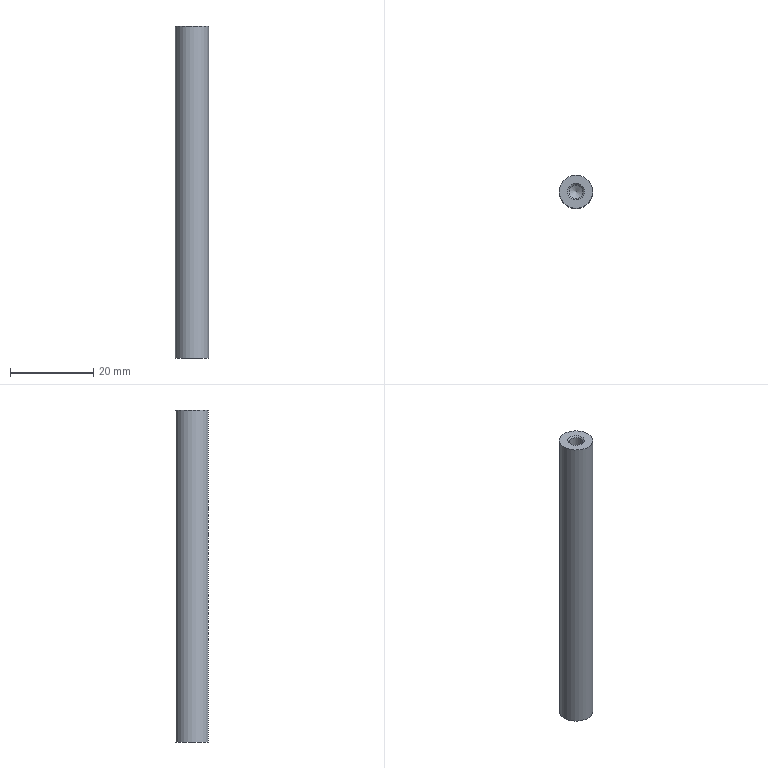Part | NX | features DATUM_CSYS 2, HOLE PACKAGE 2, SIMPLE HOLE 2, SYMBOLIC_THREAD 2, EXTRUDE 1, SKETCH 1 | 1 solid | 9 faces | box 8 x 8 x 80 mm | volume 3672 mm3 | cone 4 | cylinder 3 | plane 2 | commonest cylinder face diameters 3.3 x2 8 x1
STEP:
#1=CARTESIAN_POINT('',(4.,0.,80.));
#2=VERTEX_POINT('',#1);
#3=CARTESIAN_POINT('',(0.,0.,80.));
#4=DIRECTION('',(0.,0.,1.));
#5=DIRECTION('',(1.,0.,0.));
#6=AXIS2_PLACEMENT_3D('',#3,#4,#5);
#7=CIRCLE('',#6,4.);
#8=EDGE_CURVE('',#2,#2,#7,.T.);
#9=ORIENTED_EDGE('',*,*,#8,.F.);
#10=EDGE_LOOP('',(#9));
#11=FACE_BOUND('',#10,.T.);
#12=CARTESIAN_POINT('',(4.,0.,0.));
#13=VERTEX_POINT('',#12);
#14=CARTESIAN_POINT('',(0.,0.,0.));
#15=DIRECTION('',(0.,0.,1.));
#16=DIRECTION('',(1.,0.,0.));
#17=AXIS2_PLACEMENT_3D('',#14,#15,#16);
#18=CIRCLE('',#17,4.);
#19=EDGE_CURVE('',#13,#13,#18,.T.);
#20=ORIENTED_EDGE('',*,*,#19,.T.);
#21=EDGE_LOOP('',(#20));
#22=FACE_BOUND('',#21,.T.);
#23=CARTESIAN_POINT('',(0.,0.,80.));
#24=DIRECTION('',(0.,0.,-1.));
#25=DIRECTION('',(-1.,0.,0.));
#26=AXIS2_PLACEMENT_3D('',#23,#24,#25);
#27=CYLINDRICAL_SURFACE('',#26,4.);
#28=ADVANCED_FACE('',(#11,#22),#27,.T.);
#29=CARTESIAN_POINT('',(2.,0.,80.));
#30=VERTEX_POINT('',#29);
#31=CARTESIAN_POINT('',(0.,0.,80.));
#32=DIRECTION('',(0.,0.,1.));
#33=DIRECTION('',(1.,0.,0.));
#34=AXIS2_PLACEMENT_3D('',#31,#32,#33);
#35=CIRCLE('',#34,2.);
#36=EDGE_CURVE('',#30,#30,#35,.F.);
#37=ORIENTED_EDGE('',*,*,#36,.T.);
#38=EDGE_LOOP('',(#37));
#39=FACE_BOUND('',#38,.T.);
#40=ORIENTED_EDGE('',*,*,#8,.T.);
#41=EDGE_LOOP('',(#40));
#42=FACE_BOUND('',#41,.T.);
#43=CARTESIAN_POINT('',(0.,0.,80.));
#44=DIRECTION('',(0.,0.,1.));
#45=DIRECTION('',(1.,0.,0.));
#46=AXIS2_PLACEMENT_3D('',#43,#44,#45);
#47=PLANE('',#46);
#48=ADVANCED_FACE('',(#39,#42),#47,.T.);
#49=CARTESIAN_POINT('',(2.,0.,0.));
#50=VERTEX_POINT('',#49);
#51=CARTESIAN_POINT('',(0.,0.,0.));
#52=DIRECTION('',(0.,0.,1.));
#53=DIRECTION('',(1.,0.,0.));
#54=AXIS2_PLACEMENT_3D('',#51,#52,#53);
#55=CIRCLE('',#54,2.);
#56=EDGE_CURVE('',#50,#50,#55,.T.);
#57=ORIENTED_EDGE('',*,*,#56,.T.);
#58=EDGE_LOOP('',(#57));
#59=FACE_BOUND('',#58,.T.);
#60=ORIENTED_EDGE('',*,*,#19,.F.);
#61=EDGE_LOOP('',(#60));
#62=FACE_BOUND('',#61,.T.);
#63=CARTESIAN_POINT('',(0.,0.,0.));
#64=DIRECTION('',(0.,0.,1.));
#65=DIRECTION('',(1.,0.,0.));
#66=AXIS2_PLACEMENT_3D('',#63,#64,#65);
#67=PLANE('',#66);
#68=ADVANCED_FACE('',(#59,#62),#67,.F.);
#69=CARTESIAN_POINT('',(-1.65,0.,60.));
#70=VERTEX_POINT('',#69);
#71=CARTESIAN_POINT('',(0.,0.,60.));
#72=DIRECTION('',(0.,0.,-1.));
#73=DIRECTION('',(-1.,0.,0.));
#74=AXIS2_PLACEMENT_3D('',#71,#72,#73);
#75=CIRCLE('',#74,1.65);
#76=EDGE_CURVE('',#70,#70,#75,.F.);
#77=ORIENTED_EDGE('',*,*,#76,.T.);
#78=EDGE_LOOP('',(#77));
#79=FACE_BOUND('',#78,.T.);
#80=CARTESIAN_POINT('',(0.,0.,59.009));
#81=VERTEX_POINT('',#80);
#82=VERTEX_LOOP('',#81);
#83=FACE_BOUND('',#82,.T.);
#84=CARTESIAN_POINT('',(0.,0.,60.));
#85=DIRECTION('',(0.,0.,1.));
#86=DIRECTION('',(1.,0.,0.));
#87=AXIS2_PLACEMENT_3D('',#84,#85,#86);
#88=CONICAL_SURFACE('',#87,1.65,1.03);
#89=ADVANCED_FACE('',(#79,#83),#88,.F.);
#90=CARTESIAN_POINT('',(1.65,0.,79.65));
#91=VERTEX_POINT('',#90);
#92=CARTESIAN_POINT('',(0.,0.,79.65));
#93=DIRECTION('',(0.,0.,1.));
#94=DIRECTION('',(1.,0.,0.));
#95=AXIS2_PLACEMENT_3D('',#92,#93,#94);
#96=CIRCLE('',#95,1.65);
#97=EDGE_CURVE('',#91,#91,#96,.T.);
#98=ORIENTED_EDGE('',*,*,#97,.T.);
#99=EDGE_LOOP('',(#98));
#100=FACE_BOUND('',#99,.T.);
#101=ORIENTED_EDGE('',*,*,#76,.F.);
#102=EDGE_LOOP('',(#101));
#103=FACE_BOUND('',#102,.T.);
#104=CARTESIAN_POINT('',(0.,0.,80.));
#105=DIRECTION('',(0.,0.,-1.));
#106=DIRECTION('',(-1.,0.,0.));
#107=AXIS2_PLACEMENT_3D('',#104,#105,#106);
#108=CYLINDRICAL_SURFACE('',#107,1.65);
#109=ADVANCED_FACE('',(#100,#103),#108,.F.);
#110=ORIENTED_EDGE('',*,*,#97,.F.);
#111=EDGE_LOOP('',(#110));
#112=FACE_BOUND('',#111,.T.);
#113=ORIENTED_EDGE('',*,*,#36,.F.);
#114=EDGE_LOOP('',(#113));
#115=FACE_BOUND('',#114,.T.);
#116=CARTESIAN_POINT('',(0.,0.,80.));
#117=DIRECTION('',(0.,0.,1.));
#118=DIRECTION('',(1.,0.,0.));
#119=AXIS2_PLACEMENT_3D('',#116,#117,#118);
#120=CONICAL_SURFACE('',#119,2.,0.7854);
#121=ADVANCED_FACE('',(#112,#115),#120,.F.);
#122=CARTESIAN_POINT('',(1.65,0.,20.));
#123=VERTEX_POINT('',#122);
#124=CARTESIAN_POINT('',(0.,0.,20.));
#125=DIRECTION('',(0.,0.,1.));
#126=DIRECTION('',(1.,0.,0.));
#127=AXIS2_PLACEMENT_3D('',#124,#125,#126);
#128=CIRCLE('',#127,1.65);
#129=EDGE_CURVE('',#123,#123,#128,.F.);
#130=ORIENTED_EDGE('',*,*,#129,.T.);
#131=EDGE_LOOP('',(#130));
#132=FACE_BOUND('',#131,.T.);
#133=CARTESIAN_POINT('',(0.,0.,20.991));
#134=VERTEX_POINT('',#133);
#135=VERTEX_LOOP('',#134);
#136=FACE_BOUND('',#135,.T.);
#137=CARTESIAN_POINT('',(0.,0.,20.));
#138=DIRECTION('',(0.,0.,-1.));
#139=DIRECTION('',(-1.,0.,0.));
#140=AXIS2_PLACEMENT_3D('',#137,#138,#139);
#141=CONICAL_SURFACE('',#140,1.65,1.03);
#142=ADVANCED_FACE('',(#132,#136),#141,.F.);
#143=CARTESIAN_POINT('',(1.65,0.,0.35));
#144=VERTEX_POINT('',#143);
#145=CARTESIAN_POINT('',(0.,0.,0.35));
#146=DIRECTION('',(0.,0.,1.));
#147=DIRECTION('',(1.,0.,0.));
#148=AXIS2_PLACEMENT_3D('',#145,#146,#147);
#149=CIRCLE('',#148,1.65);
#150=EDGE_CURVE('',#144,#144,#149,.F.);
#151=ORIENTED_EDGE('',*,*,#150,.T.);
#152=EDGE_LOOP('',(#151));
#153=FACE_BOUND('',#152,.T.);
#154=ORIENTED_EDGE('',*,*,#129,.F.);
#155=EDGE_LOOP('',(#154));
#156=FACE_BOUND('',#155,.T.);
#157=CARTESIAN_POINT('',(0.,0.,0.));
#158=DIRECTION('',(0.,0.,1.));
#159=DIRECTION('',(1.,0.,0.));
#160=AXIS2_PLACEMENT_3D('',#157,#158,#159);
#161=CYLINDRICAL_SURFACE('',#160,1.65);
#162=ADVANCED_FACE('',(#153,#156),#161,.F.);
#163=ORIENTED_EDGE('',*,*,#150,.F.);
#164=EDGE_LOOP('',(#163));
#165=FACE_BOUND('',#164,.T.);
#166=ORIENTED_EDGE('',*,*,#56,.F.);
#167=EDGE_LOOP('',(#166));
#168=FACE_BOUND('',#167,.T.);
#169=CARTESIAN_POINT('',(0.,0.,0.));
#170=DIRECTION('',(0.,0.,-1.));
#171=DIRECTION('',(-1.,0.,0.));
#172=AXIS2_PLACEMENT_3D('',#169,#170,#171);
#173=CONICAL_SURFACE('',#172,2.,0.7854);
#174=ADVANCED_FACE('',(#165,#168),#173,.F.);
#175=CLOSED_SHELL('',(#28,#48,#68,#89,#109,#121,#142,#162,#174));
#176=MANIFOLD_SOLID_BREP('',#175);
#177=(LENGTH_UNIT()NAMED_UNIT(*)SI_UNIT(.MILLI.,.METRE.));
#178=UNCERTAINTY_MEASURE_WITH_UNIT(LENGTH_MEASURE(0.00001),#177,'','');
#179=(NAMED_UNIT(*)PLANE_ANGLE_UNIT()SI_UNIT($,.RADIAN.));
#180=(NAMED_UNIT(*)SI_UNIT($,.STERADIAN.)SOLID_ANGLE_UNIT());
#181=(GEOMETRIC_REPRESENTATION_CONTEXT(3)GLOBAL_UNCERTAINTY_ASSIGNED_CONTEXT((#178))GLOBAL_UNIT_ASSIGNED_CONTEXT((#177,#179,#180))REPRESENTATION_CONTEXT('',''));
#182=ADVANCED_BREP_SHAPE_REPRESENTATION('',(#176),#181);